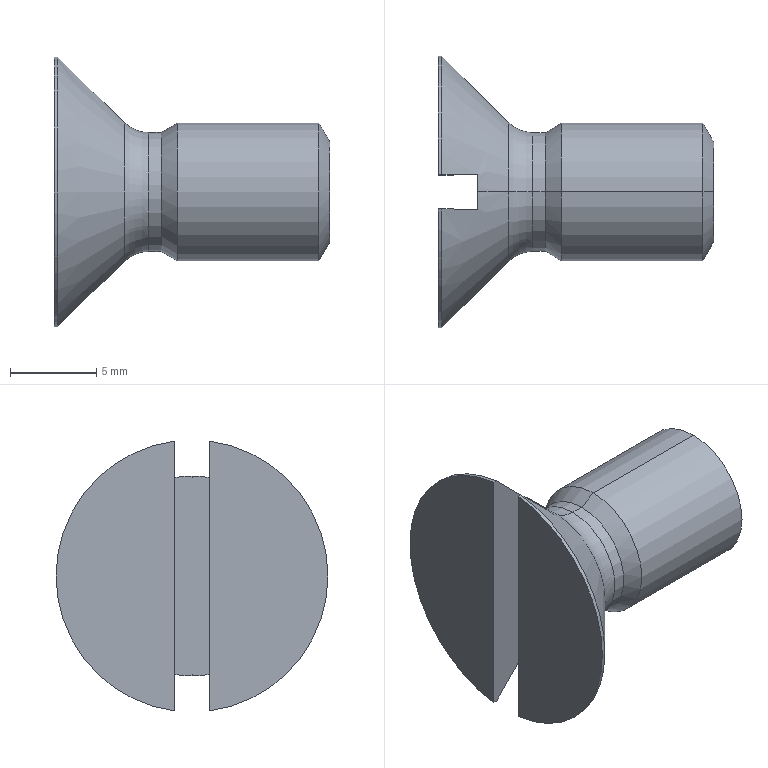Part | SolidWorks | features Chamfer 1, Cut 1, LPattern 1, RevCut 1, Revolution 1 | 1 solid | 20 faces | box 16 x 15.8 x 15.673 mm | volume 989.006 mm3 | cone 6 | cylinder 6 | plane 6 | torus 2 | commonest cylinder face diameters 6.918 x2 8 x2 15.8 x2
STEP:
#1=CARTESIAN_POINT('',(16.,0.,2.917));
#2=VERTEX_POINT('',#1);
#3=CARTESIAN_POINT('',(16.,0.,-2.917));
#4=VERTEX_POINT('',#3);
#5=CARTESIAN_POINT('',(16.,0.,0.));
#6=DIRECTION('',(-1.,0.,0.));
#7=DIRECTION('',(0.,0.,1.));
#8=AXIS2_PLACEMENT_3D('',#5,#6,#7);
#9=CIRCLE('',#8,2.917);
#10=EDGE_CURVE('',#2,#4,#9,.T.);
#11=ORIENTED_EDGE('',*,*,#10,.T.);
#12=CARTESIAN_POINT('',(15.375,0.,-4.));
#13=VERTEX_POINT('',#12);
#14=CARTESIAN_POINT('',(15.375,0.,-4.));
#15=DIRECTION('',(-0.5,0.,-0.866));
#16=VECTOR('',#15,1000.);
#17=LINE('',#14,#16);
#18=EDGE_CURVE('',#4,#13,#17,.T.);
#19=ORIENTED_EDGE('',*,*,#18,.T.);
#20=CARTESIAN_POINT('',(15.375,0.,4.));
#21=VERTEX_POINT('',#20);
#22=CARTESIAN_POINT('',(15.375,0.,0.));
#23=DIRECTION('',(-1.,0.,0.));
#24=DIRECTION('',(0.,0.,1.));
#25=AXIS2_PLACEMENT_3D('',#22,#23,#24);
#26=CIRCLE('',#25,4.);
#27=EDGE_CURVE('',#21,#13,#26,.T.);
#28=ORIENTED_EDGE('',*,*,#27,.F.);
#29=CARTESIAN_POINT('',(15.375,0.,4.));
#30=DIRECTION('',(-0.5,0.,0.866));
#31=VECTOR('',#30,1000.);
#32=LINE('',#29,#31);
#33=EDGE_CURVE('',#2,#21,#32,.T.);
#34=ORIENTED_EDGE('',*,*,#33,.F.);
#35=EDGE_LOOP('',(#11,#19,#28,#34));
#36=FACE_OUTER_BOUND('',#35,.T.);
#37=CARTESIAN_POINT('',(15.375,0.,0.));
#38=DIRECTION('',(-1.,0.,0.));
#39=DIRECTION('',(0.,0.,1.));
#40=AXIS2_PLACEMENT_3D('',#37,#38,#39);
#41=CONICAL_SURFACE('',#40,4.,1.047);
#42=ADVANCED_FACE('',(#36),#41,.T.);
#43=ORIENTED_EDGE('',*,*,#27,.T.);
#44=CARTESIAN_POINT('',(7.15,0.,-4.));
#45=VERTEX_POINT('',#44);
#46=CARTESIAN_POINT('',(0.,0.,-4.));
#47=DIRECTION('',(-1.,0.,0.));
#48=VECTOR('',#47,1000.);
#49=LINE('',#46,#48);
#50=EDGE_CURVE('',#13,#45,#49,.T.);
#51=ORIENTED_EDGE('',*,*,#50,.T.);
#52=CARTESIAN_POINT('',(7.15,0.,4.));
#53=VERTEX_POINT('',#52);
#54=CARTESIAN_POINT('',(7.15,0.,0.));
#55=DIRECTION('',(-1.,0.,0.));
#56=DIRECTION('',(0.,0.,1.));
#57=AXIS2_PLACEMENT_3D('',#54,#55,#56);
#58=CIRCLE('',#57,4.);
#59=EDGE_CURVE('',#53,#45,#58,.T.);
#60=ORIENTED_EDGE('',*,*,#59,.F.);
#61=CARTESIAN_POINT('',(0.,0.,4.));
#62=DIRECTION('',(-1.,0.,0.));
#63=VECTOR('',#62,1000.);
#64=LINE('',#61,#63);
#65=EDGE_CURVE('',#21,#53,#64,.T.);
#66=ORIENTED_EDGE('',*,*,#65,.F.);
#67=EDGE_LOOP('',(#43,#51,#60,#66));
#68=FACE_OUTER_BOUND('',#67,.T.);
#69=CARTESIAN_POINT('',(0.,0.,0.));
#70=DIRECTION('',(-1.,0.,0.));
#71=DIRECTION('',(0.,0.,1.));
#72=AXIS2_PLACEMENT_3D('',#69,#70,#71);
#73=CYLINDRICAL_SURFACE('',#72,4.);
#74=ADVANCED_FACE('',(#68),#73,.T.);
#75=CARTESIAN_POINT('',(6.213,0.,3.459));
#76=VERTEX_POINT('',#75);
#77=CARTESIAN_POINT('',(6.213,0.,-3.459));
#78=VERTEX_POINT('',#77);
#79=CARTESIAN_POINT('',(6.213,0.,0.));
#80=DIRECTION('',(-1.,0.,0.));
#81=DIRECTION('',(0.,0.,1.));
#82=AXIS2_PLACEMENT_3D('',#79,#80,#81);
#83=CIRCLE('',#82,3.459);
#84=EDGE_CURVE('',#76,#78,#83,.T.);
#85=ORIENTED_EDGE('',*,*,#84,.F.);
#86=CARTESIAN_POINT('',(7.15,0.,4.));
#87=DIRECTION('',(0.866,0.,0.5));
#88=VECTOR('',#87,1000.);
#89=LINE('',#86,#88);
#90=EDGE_CURVE('',#76,#53,#89,.T.);
#91=ORIENTED_EDGE('',*,*,#90,.T.);
#92=ORIENTED_EDGE('',*,*,#59,.T.);
#93=CARTESIAN_POINT('',(7.15,0.,-4.));
#94=DIRECTION('',(0.866,0.,-0.5));
#95=VECTOR('',#94,1000.);
#96=LINE('',#93,#95);
#97=EDGE_CURVE('',#78,#45,#96,.T.);
#98=ORIENTED_EDGE('',*,*,#97,.F.);
#99=EDGE_LOOP('',(#85,#91,#92,#98));
#100=FACE_OUTER_BOUND('',#99,.T.);
#101=CARTESIAN_POINT('',(7.15,0.,0.));
#102=DIRECTION('',(1.,0.,0.));
#103=DIRECTION('',(0.,0.,-1.));
#104=AXIS2_PLACEMENT_3D('',#101,#102,#103);
#105=CONICAL_SURFACE('',#104,4.,0.5236);
#106=ADVANCED_FACE('',(#100),#105,.T.);
#107=ORIENTED_EDGE('',*,*,#84,.T.);
#108=CARTESIAN_POINT('',(5.478,0.,-3.459));
#109=VERTEX_POINT('',#108);
#110=CARTESIAN_POINT('',(0.,0.,-3.459));
#111=DIRECTION('',(-1.,0.,0.));
#112=VECTOR('',#111,1000.);
#113=LINE('',#110,#112);
#114=EDGE_CURVE('',#78,#109,#113,.T.);
#115=ORIENTED_EDGE('',*,*,#114,.T.);
#116=CARTESIAN_POINT('',(5.478,0.,3.459));
#117=VERTEX_POINT('',#116);
#118=CARTESIAN_POINT('',(5.478,0.,0.));
#119=DIRECTION('',(-1.,0.,0.));
#120=DIRECTION('',(0.,0.,1.));
#121=AXIS2_PLACEMENT_3D('',#118,#119,#120);
#122=CIRCLE('',#121,3.459);
#123=EDGE_CURVE('',#117,#109,#122,.T.);
#124=ORIENTED_EDGE('',*,*,#123,.F.);
#125=CARTESIAN_POINT('',(0.,0.,3.459));
#126=DIRECTION('',(-1.,0.,0.));
#127=VECTOR('',#126,1000.);
#128=LINE('',#125,#127);
#129=EDGE_CURVE('',#76,#117,#128,.T.);
#130=ORIENTED_EDGE('',*,*,#129,.F.);
#131=EDGE_LOOP('',(#107,#115,#124,#130));
#132=FACE_OUTER_BOUND('',#131,.T.);
#133=CARTESIAN_POINT('',(0.,0.,0.));
#134=DIRECTION('',(-1.,0.,0.));
#135=DIRECTION('',(0.,0.,1.));
#136=AXIS2_PLACEMENT_3D('',#133,#134,#135);
#137=CYLINDRICAL_SURFACE('',#136,3.459);
#138=ADVANCED_FACE('',(#132),#137,.T.);
#139=CARTESIAN_POINT('',(4.064,0.,-4.045));
#140=VERTEX_POINT('',#139);
#141=CARTESIAN_POINT('',(4.064,0.,4.045));
#142=VERTEX_POINT('',#141);
#143=CARTESIAN_POINT('',(4.064,0.,0.));
#144=DIRECTION('',(-1.,0.,0.));
#145=DIRECTION('',(0.,0.,1.));
#146=AXIS2_PLACEMENT_3D('',#143,#144,#145);
#147=CIRCLE('',#146,4.045);
#148=EDGE_CURVE('',#140,#142,#147,.T.);
#149=ORIENTED_EDGE('',*,*,#148,.F.);
#150=CARTESIAN_POINT('',(5.478,0.,-5.459));
#151=DIRECTION('',(0.,1.,0.));
#152=DIRECTION('',(0.,0.,1.));
#153=AXIS2_PLACEMENT_3D('',#150,#151,#152);
#154=CIRCLE('',#153,2.);
#155=EDGE_CURVE('',#140,#109,#154,.T.);
#156=ORIENTED_EDGE('',*,*,#155,.T.);
#157=CARTESIAN_POINT('',(5.478,0.,0.));
#158=DIRECTION('',(-1.,0.,0.));
#159=DIRECTION('',(0.,0.,1.));
#160=AXIS2_PLACEMENT_3D('',#157,#158,#159);
#161=CIRCLE('',#160,3.459);
#162=EDGE_CURVE('',#109,#117,#161,.T.);
#163=ORIENTED_EDGE('',*,*,#162,.T.);
#164=CARTESIAN_POINT('',(5.478,0.,5.459));
#165=DIRECTION('',(0.,-1.,0.));
#166=DIRECTION('',(0.,0.,-1.));
#167=AXIS2_PLACEMENT_3D('',#164,#165,#166);
#168=CIRCLE('',#167,2.);
#169=EDGE_CURVE('',#142,#117,#168,.T.);
#170=ORIENTED_EDGE('',*,*,#169,.F.);
#171=EDGE_LOOP('',(#149,#156,#163,#170));
#172=FACE_OUTER_BOUND('',#171,.T.);
#173=CARTESIAN_POINT('',(5.478,0.,0.));
#174=DIRECTION('',(-1.,0.,0.));
#175=DIRECTION('',(0.,0.,1.));
#176=AXIS2_PLACEMENT_3D('',#173,#174,#175);
#177=TOROIDAL_SURFACE('',#176,5.459,2.);
#178=ADVANCED_FACE('',(#172),#177,.F.);
#179=CARTESIAN_POINT('',(4.064,0.,0.));
#180=DIRECTION('',(-1.,0.,0.));
#181=DIRECTION('',(0.,0.,1.));
#182=AXIS2_PLACEMENT_3D('',#179,#180,#181);
#183=CIRCLE('',#182,4.045);
#184=EDGE_CURVE('',#142,#140,#183,.T.);
#185=ORIENTED_EDGE('',*,*,#184,.T.);
#186=CARTESIAN_POINT('',(2.3,0.,-5.809));
#187=VERTEX_POINT('',#186);
#188=CARTESIAN_POINT('',(4.064,0.,-4.045));
#189=DIRECTION('',(-0.7071,0.,-0.7071));
#190=VECTOR('',#189,1000.);
#191=LINE('',#188,#190);
#192=EDGE_CURVE('',#140,#187,#191,.T.);
#193=ORIENTED_EDGE('',*,*,#192,.T.);
#194=CARTESIAN_POINT('',(2.3,1.,-5.722));
#195=VERTEX_POINT('',#194);
#196=CARTESIAN_POINT('',(2.3,0.,0.));
#197=DIRECTION('',(-1.,0.,0.));
#198=DIRECTION('',(0.,0.,1.));
#199=AXIS2_PLACEMENT_3D('',#196,#197,#198);
#200=CIRCLE('',#199,5.809);
#201=EDGE_CURVE('',#195,#187,#200,.T.);
#202=ORIENTED_EDGE('',*,*,#201,.F.);
#203=CARTESIAN_POINT('',(0.2088,1.,-7.836));
#204=VERTEX_POINT('',#203);
#205=CARTESIAN_POINT('',(2.3,1.,-5.722));
#206=CARTESIAN_POINT('',(1.604,1.,-6.428));
#207=CARTESIAN_POINT('',(0.9069,1.,-7.133));
#208=CARTESIAN_POINT('',(0.2088,1.,-7.836));
#209=B_SPLINE_CURVE_WITH_KNOTS('',3,(#205,#206,#207,#208),.UNSPECIFIED.,.F.,.F.,(4,4),(0.03148,0.03446),.UNSPECIFIED.);
#210=EDGE_CURVE('',#195,#204,#209,.T.);
#211=ORIENTED_EDGE('',*,*,#210,.T.);
#212=CARTESIAN_POINT('',(0.2088,1.,7.836));
#213=VERTEX_POINT('',#212);
#214=CARTESIAN_POINT('',(0.2088,0.,0.));
#215=DIRECTION('',(-1.,0.,0.));
#216=DIRECTION('',(0.,0.,1.));
#217=AXIS2_PLACEMENT_3D('',#214,#215,#216);
#218=CIRCLE('',#217,7.9);
#219=EDGE_CURVE('',#213,#204,#218,.T.);
#220=ORIENTED_EDGE('',*,*,#219,.F.);
#221=CARTESIAN_POINT('',(2.3,1.,5.722));
#222=VERTEX_POINT('',#221);
#223=CARTESIAN_POINT('',(0.2088,1.,7.836));
#224=CARTESIAN_POINT('',(0.9069,1.,7.133));
#225=CARTESIAN_POINT('',(1.604,1.,6.428));
#226=CARTESIAN_POINT('',(2.3,1.,5.722));
#227=B_SPLINE_CURVE_WITH_KNOTS('',3,(#223,#224,#225,#226),.UNSPECIFIED.,.F.,.F.,(4,4),(0.01339,0.01637),.UNSPECIFIED.);
#228=EDGE_CURVE('',#213,#222,#227,.T.);
#229=ORIENTED_EDGE('',*,*,#228,.T.);
#230=CARTESIAN_POINT('',(2.3,0.,5.809));
#231=VERTEX_POINT('',#230);
#232=CARTESIAN_POINT('',(2.3,0.,0.));
#233=DIRECTION('',(-1.,0.,0.));
#234=DIRECTION('',(0.,0.,1.));
#235=AXIS2_PLACEMENT_3D('',#232,#233,#234);
#236=CIRCLE('',#235,5.809);
#237=EDGE_CURVE('',#231,#222,#236,.T.);
#238=ORIENTED_EDGE('',*,*,#237,.F.);
#239=CARTESIAN_POINT('',(4.064,0.,4.045));
#240=DIRECTION('',(-0.7071,0.,0.7071));
#241=VECTOR('',#240,1000.);
#242=LINE('',#239,#241);
#243=EDGE_CURVE('',#142,#231,#242,.T.);
#244=ORIENTED_EDGE('',*,*,#243,.F.);
#245=EDGE_LOOP('',(#185,#193,#202,#211,#220,#229,#238,#244));
#246=FACE_OUTER_BOUND('',#245,.T.);
#247=CARTESIAN_POINT('',(4.064,0.,0.));
#248=DIRECTION('',(-1.,0.,0.));
#249=DIRECTION('',(0.,0.,1.));
#250=AXIS2_PLACEMENT_3D('',#247,#248,#249);
#251=CONICAL_SURFACE('',#250,4.045,0.7854);
#252=ADVANCED_FACE('',(#246),#251,.T.);
#253=CARTESIAN_POINT('',(0.,1.,7.836));
#254=VERTEX_POINT('',#253);
#255=CARTESIAN_POINT('',(0.,1.,-7.836));
#256=VERTEX_POINT('',#255);
#257=CARTESIAN_POINT('',(0.,0.,0.));
#258=DIRECTION('',(-1.,0.,0.));
#259=DIRECTION('',(0.,0.,1.));
#260=AXIS2_PLACEMENT_3D('',#257,#258,#259);
#261=CIRCLE('',#260,7.9);
#262=EDGE_CURVE('',#254,#256,#261,.T.);
#263=ORIENTED_EDGE('',*,*,#262,.T.);
#264=CARTESIAN_POINT('',(0.,1.,-7.836));
#265=DIRECTION('',(0.,0.,-1.));
#266=VECTOR('',#265,1000.);
#267=LINE('',#264,#266);
#268=EDGE_CURVE('',#254,#256,#267,.T.);
#269=ORIENTED_EDGE('',*,*,#268,.F.);
#270=EDGE_LOOP('',(#263,#269));
#271=FACE_OUTER_BOUND('',#270,.T.);
#272=CARTESIAN_POINT('',(0.,0.,0.));
#273=DIRECTION('',(1.,0.,0.));
#274=DIRECTION('',(0.,0.,-1.));
#275=AXIS2_PLACEMENT_3D('',#272,#273,#274);
#276=PLANE('',#275);
#277=ADVANCED_FACE('',(#271),#276,.F.);
#278=ORIENTED_EDGE('',*,*,#219,.T.);
#279=CARTESIAN_POINT('',(2.3,1.,-7.836));
#280=DIRECTION('',(-1.,0.,0.));
#281=VECTOR('',#280,1000.);
#282=LINE('',#279,#281);
#283=EDGE_CURVE('',#204,#256,#282,.T.);
#284=ORIENTED_EDGE('',*,*,#283,.T.);
#285=ORIENTED_EDGE('',*,*,#262,.F.);
#286=CARTESIAN_POINT('',(2.3,1.,7.836));
#287=DIRECTION('',(-1.,0.,0.));
#288=VECTOR('',#287,1000.);
#289=LINE('',#286,#288);
#290=EDGE_CURVE('',#213,#254,#289,.T.);
#291=ORIENTED_EDGE('',*,*,#290,.F.);
#292=EDGE_LOOP('',(#278,#284,#285,#291));
#293=FACE_OUTER_BOUND('',#292,.T.);
#294=CARTESIAN_POINT('',(0.,0.,0.));
#295=DIRECTION('',(-1.,0.,0.));
#296=DIRECTION('',(0.,0.,1.));
#297=AXIS2_PLACEMENT_3D('',#294,#295,#296);
#298=CYLINDRICAL_SURFACE('',#297,7.9);
#299=ADVANCED_FACE('',(#293),#298,.T.);
#300=CARTESIAN_POINT('',(0.,-1.,-7.836));
#301=VERTEX_POINT('',#300);
#302=CARTESIAN_POINT('',(0.,-1.,7.836));
#303=VERTEX_POINT('',#302);
#304=CARTESIAN_POINT('',(0.,0.,0.));
#305=DIRECTION('',(-1.,0.,0.));
#306=DIRECTION('',(0.,0.,1.));
#307=AXIS2_PLACEMENT_3D('',#304,#305,#306);
#308=CIRCLE('',#307,7.9);
#309=EDGE_CURVE('',#301,#303,#308,.T.);
#310=ORIENTED_EDGE('',*,*,#309,.T.);
#311=CARTESIAN_POINT('',(0.,-1.,-7.836));
#312=DIRECTION('',(0.,0.,1.));
#313=VECTOR('',#312,1000.);
#314=LINE('',#311,#313);
#315=EDGE_CURVE('',#301,#303,#314,.T.);
#316=ORIENTED_EDGE('',*,*,#315,.F.);
#317=EDGE_LOOP('',(#310,#316));
#318=FACE_OUTER_BOUND('',#317,.T.);
#319=CARTESIAN_POINT('',(0.,0.,0.));
#320=DIRECTION('',(1.,0.,0.));
#321=DIRECTION('',(0.,0.,-1.));
#322=AXIS2_PLACEMENT_3D('',#319,#320,#321);
#323=PLANE('',#322);
#324=ADVANCED_FACE('',(#318),#323,.F.);
#325=CARTESIAN_POINT('',(0.2088,-1.,-7.836));
#326=VERTEX_POINT('',#325);
#327=CARTESIAN_POINT('',(0.2088,-1.,7.836));
#328=VERTEX_POINT('',#327);
#329=CARTESIAN_POINT('',(0.2088,0.,0.));
#330=DIRECTION('',(-1.,0.,0.));
#331=DIRECTION('',(0.,0.,1.));
#332=AXIS2_PLACEMENT_3D('',#329,#330,#331);
#333=CIRCLE('',#332,7.9);
#334=EDGE_CURVE('',#326,#328,#333,.T.);
#335=ORIENTED_EDGE('',*,*,#334,.T.);
#336=CARTESIAN_POINT('',(2.3,-1.,7.836));
#337=DIRECTION('',(-1.,0.,0.));
#338=VECTOR('',#337,1000.);
#339=LINE('',#336,#338);
#340=EDGE_CURVE('',#328,#303,#339,.T.);
#341=ORIENTED_EDGE('',*,*,#340,.T.);
#342=ORIENTED_EDGE('',*,*,#309,.F.);
#343=CARTESIAN_POINT('',(2.3,-1.,-7.836));
#344=DIRECTION('',(-1.,0.,0.));
#345=VECTOR('',#344,1000.);
#346=LINE('',#343,#345);
#347=EDGE_CURVE('',#326,#301,#346,.T.);
#348=ORIENTED_EDGE('',*,*,#347,.F.);
#349=EDGE_LOOP('',(#335,#341,#342,#348));
#350=FACE_OUTER_BOUND('',#349,.T.);
#351=CARTESIAN_POINT('',(0.,0.,0.));
#352=DIRECTION('',(-1.,0.,0.));
#353=DIRECTION('',(0.,0.,1.));
#354=AXIS2_PLACEMENT_3D('',#351,#352,#353);
#355=CYLINDRICAL_SURFACE('',#354,7.9);
#356=ADVANCED_FACE('',(#350),#355,.T.);
#357=ORIENTED_EDGE('',*,*,#192,.F.);
#358=ORIENTED_EDGE('',*,*,#148,.T.);
#359=ORIENTED_EDGE('',*,*,#243,.T.);
#360=CARTESIAN_POINT('',(2.3,-1.,5.722));
#361=VERTEX_POINT('',#360);
#362=CARTESIAN_POINT('',(2.3,0.,0.));
#363=DIRECTION('',(-1.,0.,0.));
#364=DIRECTION('',(0.,0.,1.));
#365=AXIS2_PLACEMENT_3D('',#362,#363,#364);
#366=CIRCLE('',#365,5.809);
#367=EDGE_CURVE('',#361,#231,#366,.T.);
#368=ORIENTED_EDGE('',*,*,#367,.F.);
#369=CARTESIAN_POINT('',(2.3,-1.,5.722));
#370=CARTESIAN_POINT('',(1.604,-1.,6.428));
#371=CARTESIAN_POINT('',(0.9069,-1.,7.133));
#372=CARTESIAN_POINT('',(0.2088,-1.,7.836));
#373=B_SPLINE_CURVE_WITH_KNOTS('',3,(#369,#370,#371,#372),.UNSPECIFIED.,.F.,.F.,(4,4),(0.03148,0.03446),.UNSPECIFIED.);
#374=EDGE_CURVE('',#361,#328,#373,.T.);
#375=ORIENTED_EDGE('',*,*,#374,.T.);
#376=ORIENTED_EDGE('',*,*,#334,.F.);
#377=CARTESIAN_POINT('',(2.3,-1.,-5.722));
#378=VERTEX_POINT('',#377);
#379=CARTESIAN_POINT('',(0.2088,-1.,-7.836));
#380=CARTESIAN_POINT('',(0.9069,-1.,-7.133));
#381=CARTESIAN_POINT('',(1.604,-1.,-6.428));
#382=CARTESIAN_POINT('',(2.3,-1.,-5.722));
#383=B_SPLINE_CURVE_WITH_KNOTS('',3,(#379,#380,#381,#382),.UNSPECIFIED.,.F.,.F.,(4,4),(0.01339,0.01637),.UNSPECIFIED.);
#384=EDGE_CURVE('',#326,#378,#383,.T.);
#385=ORIENTED_EDGE('',*,*,#384,.T.);
#386=CARTESIAN_POINT('',(2.3,0.,0.));
#387=DIRECTION('',(-1.,0.,0.));
#388=DIRECTION('',(0.,0.,1.));
#389=AXIS2_PLACEMENT_3D('',#386,#387,#388);
#390=CIRCLE('',#389,5.809);
#391=EDGE_CURVE('',#187,#378,#390,.T.);
#392=ORIENTED_EDGE('',*,*,#391,.F.);
#393=EDGE_LOOP('',(#357,#358,#359,#368,#375,#376,#385,#392));
#394=FACE_OUTER_BOUND('',#393,.T.);
#395=CARTESIAN_POINT('',(4.064,0.,0.));
#396=DIRECTION('',(-1.,0.,0.));
#397=DIRECTION('',(0.,0.,1.));
#398=AXIS2_PLACEMENT_3D('',#395,#396,#397);
#399=CONICAL_SURFACE('',#398,4.045,0.7854);
#400=ADVANCED_FACE('',(#394),#399,.T.);
#401=ORIENTED_EDGE('',*,*,#155,.F.);
#402=ORIENTED_EDGE('',*,*,#184,.F.);
#403=ORIENTED_EDGE('',*,*,#169,.T.);
#404=ORIENTED_EDGE('',*,*,#123,.T.);
#405=EDGE_LOOP('',(#401,#402,#403,#404));
#406=FACE_OUTER_BOUND('',#405,.T.);
#407=CARTESIAN_POINT('',(5.478,0.,0.));
#408=DIRECTION('',(-1.,0.,0.));
#409=DIRECTION('',(0.,0.,1.));
#410=AXIS2_PLACEMENT_3D('',#407,#408,#409);
#411=TOROIDAL_SURFACE('',#410,5.459,2.);
#412=ADVANCED_FACE('',(#406),#411,.F.);
#413=ORIENTED_EDGE('',*,*,#114,.F.);
#414=CARTESIAN_POINT('',(6.213,0.,0.));
#415=DIRECTION('',(-1.,0.,0.));
#416=DIRECTION('',(0.,0.,1.));
#417=AXIS2_PLACEMENT_3D('',#414,#415,#416);
#418=CIRCLE('',#417,3.459);
#419=EDGE_CURVE('',#78,#76,#418,.T.);
#420=ORIENTED_EDGE('',*,*,#419,.T.);
#421=ORIENTED_EDGE('',*,*,#129,.T.);
#422=ORIENTED_EDGE('',*,*,#162,.F.);
#423=EDGE_LOOP('',(#413,#420,#421,#422));
#424=FACE_OUTER_BOUND('',#423,.T.);
#425=CARTESIAN_POINT('',(0.,0.,0.));
#426=DIRECTION('',(-1.,0.,0.));
#427=DIRECTION('',(0.,0.,1.));
#428=AXIS2_PLACEMENT_3D('',#425,#426,#427);
#429=CYLINDRICAL_SURFACE('',#428,3.459);
#430=ADVANCED_FACE('',(#424),#429,.T.);
#431=ORIENTED_EDGE('',*,*,#90,.F.);
#432=ORIENTED_EDGE('',*,*,#419,.F.);
#433=ORIENTED_EDGE('',*,*,#97,.T.);
#434=CARTESIAN_POINT('',(7.15,0.,0.));
#435=DIRECTION('',(-1.,0.,0.));
#436=DIRECTION('',(0.,0.,1.));
#437=AXIS2_PLACEMENT_3D('',#434,#435,#436);
#438=CIRCLE('',#437,4.);
#439=EDGE_CURVE('',#45,#53,#438,.T.);
#440=ORIENTED_EDGE('',*,*,#439,.T.);
#441=EDGE_LOOP('',(#431,#432,#433,#440));
#442=FACE_OUTER_BOUND('',#441,.T.);
#443=CARTESIAN_POINT('',(7.15,0.,0.));
#444=DIRECTION('',(1.,0.,0.));
#445=DIRECTION('',(0.,0.,-1.));
#446=AXIS2_PLACEMENT_3D('',#443,#444,#445);
#447=CONICAL_SURFACE('',#446,4.,0.5236);
#448=ADVANCED_FACE('',(#442),#447,.T.);
#449=ORIENTED_EDGE('',*,*,#50,.F.);
#450=CARTESIAN_POINT('',(15.375,0.,0.));
#451=DIRECTION('',(-1.,0.,0.));
#452=DIRECTION('',(0.,0.,1.));
#453=AXIS2_PLACEMENT_3D('',#450,#451,#452);
#454=CIRCLE('',#453,4.);
#455=EDGE_CURVE('',#13,#21,#454,.T.);
#456=ORIENTED_EDGE('',*,*,#455,.T.);
#457=ORIENTED_EDGE('',*,*,#65,.T.);
#458=ORIENTED_EDGE('',*,*,#439,.F.);
#459=EDGE_LOOP('',(#449,#456,#457,#458));
#460=FACE_OUTER_BOUND('',#459,.T.);
#461=CARTESIAN_POINT('',(0.,0.,0.));
#462=DIRECTION('',(-1.,0.,0.));
#463=DIRECTION('',(0.,0.,1.));
#464=AXIS2_PLACEMENT_3D('',#461,#462,#463);
#465=CYLINDRICAL_SURFACE('',#464,4.);
#466=ADVANCED_FACE('',(#460),#465,.T.);
#467=ORIENTED_EDGE('',*,*,#290,.T.);
#468=ORIENTED_EDGE('',*,*,#268,.T.);
#469=ORIENTED_EDGE('',*,*,#283,.F.);
#470=ORIENTED_EDGE('',*,*,#210,.F.);
#471=CARTESIAN_POINT('',(2.3,1.,-7.836));
#472=DIRECTION('',(0.,0.,-1.));
#473=VECTOR('',#472,1000.);
#474=LINE('',#471,#473);
#475=EDGE_CURVE('',#222,#195,#474,.T.);
#476=ORIENTED_EDGE('',*,*,#475,.F.);
#477=ORIENTED_EDGE('',*,*,#228,.F.);
#478=EDGE_LOOP('',(#467,#468,#469,#470,#476,#477));
#479=FACE_OUTER_BOUND('',#478,.T.);
#480=CARTESIAN_POINT('',(2.3,1.,-7.836));
#481=DIRECTION('',(0.,1.,0.));
#482=DIRECTION('',(0.,0.,1.));
#483=AXIS2_PLACEMENT_3D('',#480,#481,#482);
#484=PLANE('',#483);
#485=ADVANCED_FACE('',(#479),#484,.F.);
#486=ORIENTED_EDGE('',*,*,#347,.T.);
#487=ORIENTED_EDGE('',*,*,#315,.T.);
#488=ORIENTED_EDGE('',*,*,#340,.F.);
#489=ORIENTED_EDGE('',*,*,#374,.F.);
#490=CARTESIAN_POINT('',(2.3,-1.,-7.836));
#491=DIRECTION('',(0.,0.,1.));
#492=VECTOR('',#491,1000.);
#493=LINE('',#490,#492);
#494=EDGE_CURVE('',#378,#361,#493,.T.);
#495=ORIENTED_EDGE('',*,*,#494,.F.);
#496=ORIENTED_EDGE('',*,*,#384,.F.);
#497=EDGE_LOOP('',(#486,#487,#488,#489,#495,#496));
#498=FACE_OUTER_BOUND('',#497,.T.);
#499=CARTESIAN_POINT('',(2.3,-1.,-7.836));
#500=DIRECTION('',(0.,-1.,0.));
#501=DIRECTION('',(0.,0.,-1.));
#502=AXIS2_PLACEMENT_3D('',#499,#500,#501);
#503=PLANE('',#502);
#504=ADVANCED_FACE('',(#498),#503,.F.);
#505=ORIENTED_EDGE('',*,*,#201,.T.);
#506=ORIENTED_EDGE('',*,*,#391,.T.);
#507=ORIENTED_EDGE('',*,*,#494,.T.);
#508=ORIENTED_EDGE('',*,*,#367,.T.);
#509=ORIENTED_EDGE('',*,*,#237,.T.);
#510=ORIENTED_EDGE('',*,*,#475,.T.);
#511=EDGE_LOOP('',(#505,#506,#507,#508,#509,#510));
#512=FACE_OUTER_BOUND('',#511,.T.);
#513=CARTESIAN_POINT('',(2.3,0.,0.));
#514=DIRECTION('',(-1.,0.,0.));
#515=DIRECTION('',(0.,0.,1.));
#516=AXIS2_PLACEMENT_3D('',#513,#514,#515);
#517=PLANE('',#516);
#518=ADVANCED_FACE('',(#512),#517,.T.);
#519=ORIENTED_EDGE('',*,*,#18,.F.);
#520=CARTESIAN_POINT('',(16.,0.,0.));
#521=DIRECTION('',(-1.,0.,0.));
#522=DIRECTION('',(0.,0.,1.));
#523=AXIS2_PLACEMENT_3D('',#520,#521,#522);
#524=CIRCLE('',#523,2.917);
#525=EDGE_CURVE('',#4,#2,#524,.T.);
#526=ORIENTED_EDGE('',*,*,#525,.T.);
#527=ORIENTED_EDGE('',*,*,#33,.T.);
#528=ORIENTED_EDGE('',*,*,#455,.F.);
#529=EDGE_LOOP('',(#519,#526,#527,#528));
#530=FACE_OUTER_BOUND('',#529,.T.);
#531=CARTESIAN_POINT('',(15.375,0.,0.));
#532=DIRECTION('',(-1.,0.,0.));
#533=DIRECTION('',(0.,0.,1.));
#534=AXIS2_PLACEMENT_3D('',#531,#532,#533);
#535=CONICAL_SURFACE('',#534,4.,1.047);
#536=ADVANCED_FACE('',(#530),#535,.T.);
#537=ORIENTED_EDGE('',*,*,#10,.F.);
#538=ORIENTED_EDGE('',*,*,#525,.F.);
#539=EDGE_LOOP('',(#537,#538));
#540=FACE_OUTER_BOUND('',#539,.T.);
#541=CARTESIAN_POINT('',(16.,4.,0.));
#542=DIRECTION('',(-1.,0.,0.));
#543=DIRECTION('',(0.,0.,1.));
#544=AXIS2_PLACEMENT_3D('',#541,#542,#543);
#545=PLANE('',#544);
#546=ADVANCED_FACE('',(#540),#545,.F.);
#547=CLOSED_SHELL('',(#42,#74,#106,#138,#178,#252,#277,#299,#324,#356,#400,#412,#430,#448,#466,#485,#504,#518,#536,#546));
#548=MANIFOLD_SOLID_BREP('',#547);
#549=CARTESIAN_POINT('',(0.,0.,0.));
#550=DIRECTION('',(0.,0.,1.));
#551=DIRECTION('',(1.,0.,0.));
#552=AXIS2_PLACEMENT_3D('',#549,#550,#551);
#553=(LENGTH_UNIT()NAMED_UNIT(*)SI_UNIT(.MILLI.,.METRE.));
#554=UNCERTAINTY_MEASURE_WITH_UNIT(LENGTH_MEASURE(0.00001),#553,'','');
#555=(NAMED_UNIT(*)PLANE_ANGLE_UNIT()SI_UNIT($,.RADIAN.));
#556=(NAMED_UNIT(*)SI_UNIT($,.STERADIAN.)SOLID_ANGLE_UNIT());
#557=(GEOMETRIC_REPRESENTATION_CONTEXT(3)GLOBAL_UNCERTAINTY_ASSIGNED_CONTEXT((#554))GLOBAL_UNIT_ASSIGNED_CONTEXT((#553,#555,#556))REPRESENTATION_CONTEXT('',''));
#558=ADVANCED_BREP_SHAPE_REPRESENTATION('',(#548,#552),#557);